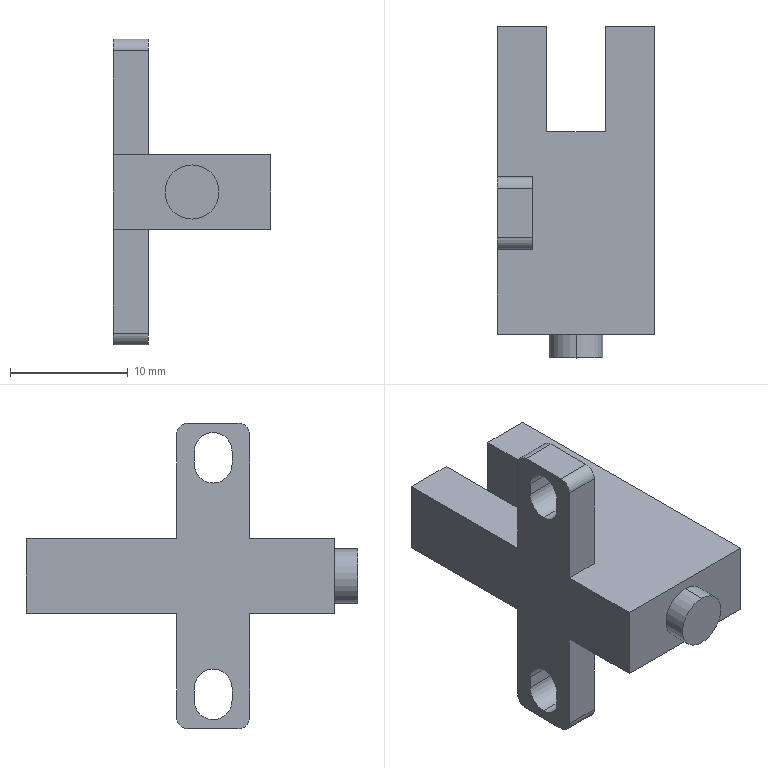Part | STEP file | 001-010-SPX303 (Omron) | 1 solid | 35 faces | box 13.4 x 28.2 x 26 mm | volume 2270 mm3 | plane 23 | cylinder 12 | commonest cylinder face diameters 3.2 x6 2 x4 4.6 x2